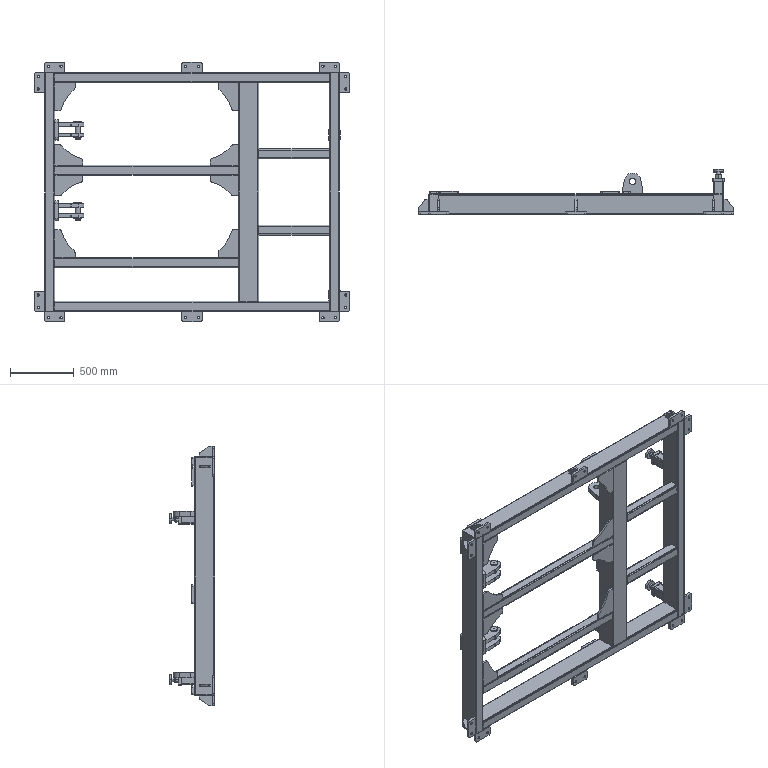Part | SolidWorks | 69 solids | 928 faces | box 2480 x 355 x 2040 mm | volume 44569591 mm3 | plane 480 | cylinder 392 | cone 56 | commonest cylinder face diameters 20 x84 14 x64 40 x64 10 x60 18 x40 30 x28